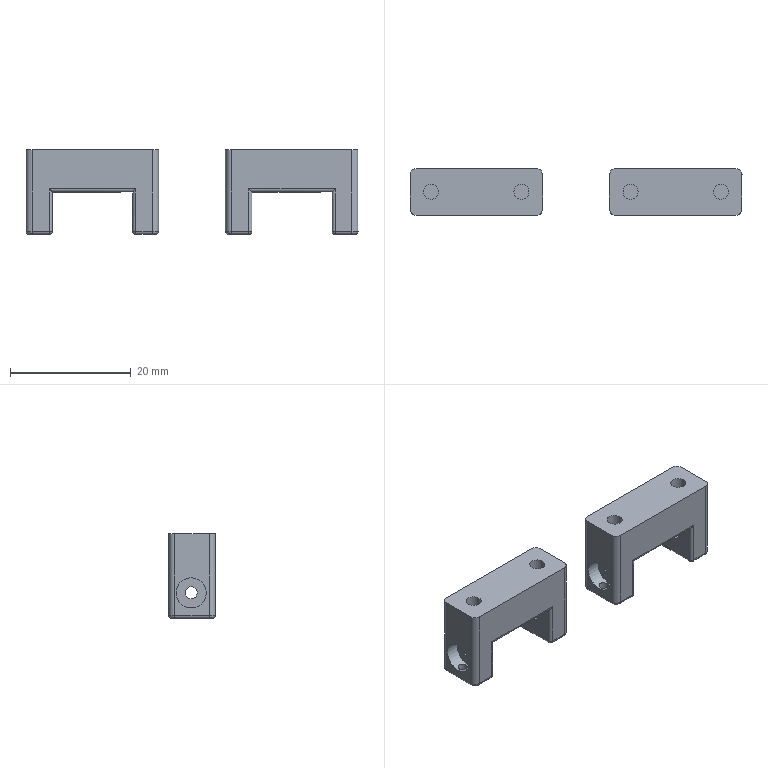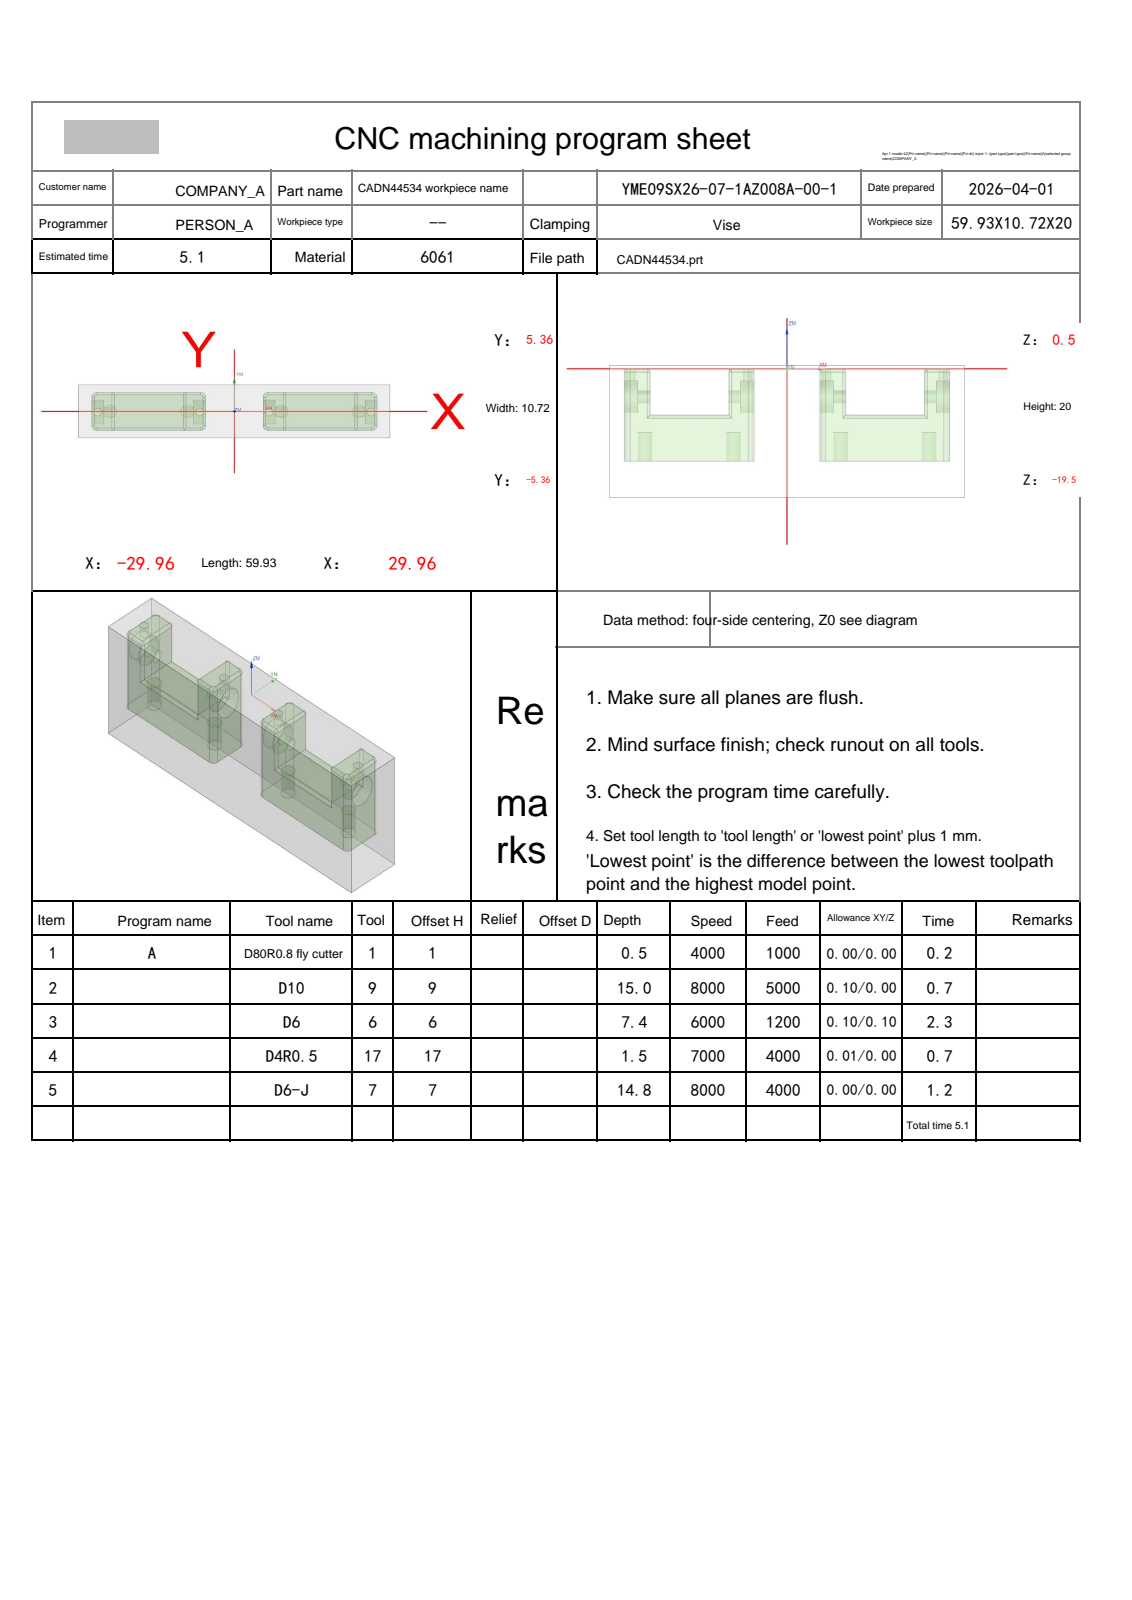NC program | NX | posted by the shop | part box 54.928 x 7.717 x 14 mm
Lines 1616 to 2983 of 13497:
N4 T17 M06
(D4R0.5  D=4. R=0.5 H=17 ce=0.01 di=0.00)
G00 G90 G54 X-28.601 Y-1.585 M03 S7000
G43 H17 Z20.
M08
Z1.5
G01 X-28.598 Y-.024 Z1.418 F4000.
X-28.602 Y2.988 Z1.26
X-28.542 Y3.372 Z1.24
X-28.414 Y3.739 Z1.22
X-28.222 Y4.077 Z1.199
X-27.973 Y4.375 Z1.179
X-27.675 Y4.624 Z1.159
X-27.337 Y4.816 Z1.138
X-26.97 Y4.944 Z1.118
X-26.586 Y5.005 Z1.097
X-23.674 Y5.001 Z.945
X-23.497 Y5.006 Z.936
X-23.368 Y4.999 Z.929
X-23.055 Y4.926 Z.912
X-22.762 Y4.795 Z.895
X-22.499 Y4.608 Z.878
X-22.278 Y4.375 Z.861
X-22.106 Y4.103 Z.845
X-21.99 Y3.804 Z.828
X-21.934 Y3.487 Z.811
Y3.358 Z.804
X-21.944 Y3.286 Z.8
X-21.943 Y-3.286 Z.456
X-21.936 Y-3.436 Z.448
X-21.942 Y-3.565 Z.441
X-22.013 Y-3.88 Z.424
X-22.144 Y-4.175 Z.407
X-22.33 Y-4.439 Z.39
X-22.564 Y-4.662 Z.373
X-22.836 Y-4.835 Z.357
X-23.137 Y-4.952 Z.34
X-23.455 Y-5.008 Z.323
X-23.584 Z.316
X-23.674 Y-5.001 Z.311
X-26.474 Y-5. Z.164
X-26.62 Y-4.999 Z.157
X-26.995 Y-4.938 Z.137
X-27.352 Y-4.812 Z.117
X-27.682 Y-4.625 Z.097
X-27.974 Y-4.383 Z.077
X-28.219 Y-4.093 Z.057
X-28.409 Y-3.765 Z.038
X-28.537 Y-3.408 Z.018
X-28.601 Y-3.034 Z-.002
X-28.603 Y-2.888 Z-.01
G03 X-28.6 Y.376 I-1732.562 J3.264
X-28.602 Y2.841 I-1732.565 J0.0
G01 Y2.844
G02 X-26.441 Y5.004 I2.161 J0.0
G01 X-26.439
X-23.674 Y5.001
X-23.497 Y5.006
G02 X-21.934 Y3.358 I-.087 J-1.648
G01 X-21.944 Y3.286
X-21.943 Y-3.286
X-21.936 Y-3.436
G02 X-23.584 Y-5.008 I-1.648 J.078
G01 X-23.674 Y-5.001
X-26.474 Y-5.
G02 X-28.603 Y-2.888 I.01 J2.14
G01 X-28.613 Y-2.871
Y-2.853
X-28.616 Y-2.146
X-28.618 Y-1.438 Z-.011
Y-1.085
X-28.621 Y-.731
X-28.618 Y-.377
X-28.609 Y-.024
X-28.623 Y.156
X-28.624 Y.336 Z-.012
Y.516
Y.695
X-28.625 Y1.055
X-28.626 Y1.414
X-28.628 Y2.133 Z-.013
X-28.631 Y2.851
Y2.921
X-28.628 Y2.99
X-28.622 Y3.058
X-28.614 Y3.127
X-28.592 Y3.269
X-28.561 Y3.409
X-28.52 Y3.547
X-28.471 Y3.683
X-28.412 Y3.814
X-28.345 Y3.941 Z-.014
X-28.269 Y4.064
X-28.186 Y4.181
X-28.094 Y4.293
X-27.996 Y4.399
X-27.891 Y4.496
X-27.779 Y4.588
X-27.662 Y4.671
X-27.539 Y4.746
X-27.412 Y4.814
X-27.281 Y4.873
X-27.214 Y4.899
X-27.146 Y4.923
X-27.077 Y4.945
X-27.008 Y4.964
X-26.868 Y4.997 Z-.015
X-26.726 Y5.02
X-26.589 Y5.033
X-26.452 Y5.038
X-25.063 Y5.042 Z-.016
X-23.674 Y5.047
X-23.628
X-23.583 Y5.048
X-23.539 Y5.047
X-23.495 Y5.046
X-23.431 Y5.041
X-23.367 Y5.034
X-23.303 Y5.025
X-23.24 Y5.013
X-23.178 Y4.999 Z-.017
X-23.116 Y4.983
X-23.054 Y4.964
X-22.994 Y4.943
X-22.934 Y4.92
X-22.875 Y4.894
X-22.817 Y4.866
X-22.76 Y4.836
X-22.705 Y4.804
X-22.651 Y4.77
X-22.598 Y4.734
X-22.546 Y4.696
X-22.496 Y4.655
X-22.447 Y4.613
X-22.4 Y4.569
X-22.355 Y4.524
X-22.312 Y4.476
X-22.27 Y4.427
X-22.23 Y4.377
X-22.192 Y4.325
X-22.157 Y4.272
X-22.123 Y4.217
X-22.091 Y4.161
X-22.062 Y4.104
X-22.034 Y4.046
X-22.009 Y3.986
X-21.986 Y3.926
X-21.966 Y3.865
X-21.948 Y3.804
X-21.932 Y3.741 Z-.018
X-21.918 Y3.678
X-21.907 Y3.615
X-21.898 Y3.551
X-21.892 Y3.487
X-21.888 Y3.423
X-21.887 Y3.358
Y3.322
X-21.888 Y3.286
X-21.882 Y1.643 Z-.019
X-21.879 Y0.0 Z-.02
X-21.874 Y-1.643
X-21.87 Y-3.286 Z-.021
X-21.869 Y-3.323
Y-3.359
Y-3.399
X-21.871 Y-3.439
X-21.875 Y-3.505
X-21.882 Y-3.569
X-21.89 Y-3.634
X-21.902 Y-3.698
X-21.916 Y-3.762 Z-.022
X-21.933 Y-3.826
X-21.951 Y-3.888
X-21.973 Y-3.95
X-21.996 Y-4.011
X-22.022 Y-4.071
X-22.05 Y-4.13
X-22.081 Y-4.188
X-22.113 Y-4.245
X-22.148 Y-4.3
X-22.184 Y-4.354
X-22.223 Y-4.407
X-22.264 Y-4.458
X-22.307 Y-4.508
X-22.351 Y-4.556
X-22.398 Y-4.602
X-22.446 Y-4.646
X-22.496 Y-4.689
X-22.547 Y-4.729
X-22.6 Y-4.768
X-22.654 Y-4.805
X-22.71 Y-4.839
X-22.767 Y-4.872
X-22.825 Y-4.902
X-22.884 Y-4.93
X-22.944 Y-4.955
X-23.006 Y-4.979
X-23.068 Y-5.
X-23.13 Y-5.018 Z-.023
X-23.194 Y-5.034
X-23.258 Y-5.048
X-23.323 Y-5.06
X-23.388 Y-5.069
X-23.453 Y-5.075
X-23.52 Y-5.079
X-23.587 Y-5.08
X-23.63
X-23.674
X-25.066 Y-5.082 Z-.024
X-26.475 Y-5.084
X-26.547
X-26.619 Y-5.081
X-26.69 Y-5.075
X-26.762 Y-5.065
X-26.833 Y-5.055
X-26.904 Y-5.042 Z-.025
X-26.974 Y-5.027
X-27.044 Y-5.009
X-27.182 Y-4.968
X-27.317 Y-4.917
X-27.448 Y-4.858
X-27.575 Y-4.79
X-27.638 Y-4.754
X-27.698 Y-4.715
X-27.758 Y-4.674
X-27.816 Y-4.631
X-27.928 Y-4.541
X-28.034 Y-4.443
X-28.133 Y-4.338
X-28.225 Y-4.227
X-28.269 Y-4.17
X-28.311 Y-4.111
X-28.35 Y-4.051
X-28.387 Y-3.989 Z-.026
X-28.424 Y-3.927
X-28.457 Y-3.863
X-28.489 Y-3.798
X-28.518 Y-3.732
X-28.57 Y-3.597
X-28.614 Y-3.46
X-28.633 Y-3.39
X-28.649 Y-3.319
X-28.663 Y-3.249
X-28.674 Y-3.177
X-28.684 Y-3.106
X-28.692 Y-3.034
X-28.696 Y-2.962
X-28.693 Y-2.889
X-28.698 Y-2.888
Y-2.87
X-28.699 Y-2.853
X-28.704 Y-1.427 Z-.027
X-28.708 Y-.001 Z-.028
X-28.713 Y1.425 Z-.029
X-28.717 Y2.852 Z-.03
X-28.718 Y2.869
X-28.717 Y2.887
X-28.711 Y3.017 Z-.031
X-28.696 Y3.147
X-28.685 Y3.22
X-28.672 Y3.293
X-28.657 Y3.366
X-28.639 Y3.437
X-28.619 Y3.509
X-28.597 Y3.579
X-28.572 Y3.649
X-28.545 Y3.718
X-28.484 Y3.853
X-28.414 Y3.984
X-28.377 Y4.048
X-28.337 Y4.111
X-28.295 Y4.171
X-28.25 Y4.231
X-28.157 Y4.346 Z-.032
X-28.056 Y4.454
X-28.002 Y4.506
X-27.947 Y4.556
X-27.891 Y4.604
X-27.832 Y4.65
X-27.773 Y4.694
X-27.712 Y4.737
X-27.65 Y4.777
X-27.586 Y4.815
X-27.455 Y4.885
X-27.32 Y4.946
X-27.251 Y4.973
X-27.181 Y4.998
X-27.111 Y5.021 Z-.033
X-27.039 Y5.04
X-26.967 Y5.059
X-26.895 Y5.074
X-26.822 Y5.087
X-26.749 Y5.098
X-26.68 Y5.108
X-26.611 Y5.115
X-26.543 Y5.12
X-26.474 Y5.122
X-26.463
X-26.453
X-25.063 Y5.126 Z-.034
X-23.674 Y5.13 Z-.035
X-23.63 Y5.131
X-23.586
X-23.458 Y5.127
X-23.331 Y5.113
X-23.207 Y5.091
X-23.084 Y5.06
X-22.964 Y5.021 Z-.036
X-22.847 Y4.972
X-22.733 Y4.916
X-22.624 Y4.852
X-22.52 Y4.78
X-22.421 Y4.7
X-22.328 Y4.614
X-22.241 Y4.522
X-22.161 Y4.423
X-22.089 Y4.319
X-22.024 Y4.21 Z-.037
X-21.967 Y4.097
X-21.918 Y3.98
X-21.877 Y3.859
X-21.846 Y3.736
X-21.823 Y3.612
X-21.809 Y3.485
X-21.804 Y3.358
X-21.801 Y1.679 Z-.038
X-21.796 Y0.0 Z-.04
X-21.792 Y-1.679 Z-.041
X-21.787 Y-3.358 Z-.042
X-21.791 Y-3.487
X-21.805 Y-3.614
X-21.827 Y-3.74
X-21.859 Y-3.865 Z-.043
X-21.899 Y-3.987
X-21.948 Y-4.105
X-22.005 Y-4.221
X-22.07 Y-4.331
X-22.143 Y-4.437
X-22.223 Y-4.537
X-22.311 Y-4.631
X-22.405 Y-4.719
X-22.504 Y-4.8
X-22.61 Y-4.874
X-22.72 Y-4.94 Z-.044
X-22.835 Y-4.997
X-22.954 Y-5.047
X-23.076 Y-5.088
X-23.201 Y-5.12
X-23.327 Y-5.143
X-23.457 Y-5.157
X-23.587 Y-5.162
X-23.63 Y-5.16
X-23.673
X-25.065 Y-5.163 Z-.045
X-26.474 Y-5.167 Z-.046
X-26.545 Y-5.165
X-26.616 Y-5.16
X-26.686 Y-5.153 Z-.047
X-26.756 Y-5.144
X-26.83 Y-5.132
X-26.904 Y-5.12
X-26.977 Y-5.104
X-27.05 Y-5.086
X-27.193 Y-5.044
X-27.334 Y-4.993
X-27.471 Y-4.932
X-27.603 Y-4.862
X-27.668 Y-4.824
X-27.731 Y-4.785
X-27.793 Y-4.743
X-27.854 Y-4.698
X-27.971 Y-4.605 Z-.048
X-28.081 Y-4.504
X-28.185 Y-4.395
X-28.281 Y-4.28
X-28.326 Y-4.22
X-28.37 Y-4.16
X-28.412 Y-4.097
X-28.45 Y-4.033
X-28.488 Y-3.968
X-28.523 Y-3.902
X-28.556 Y-3.834
X-28.587 Y-3.766
X-28.641 Y-3.626
X-28.688 Y-3.483 Z-.049
X-28.706 Y-3.411
X-28.724 Y-3.338
X-28.738 Y-3.264
X-28.75 Y-3.19
X-28.762 Y-3.116
X-28.771 Y-3.041
X-28.776 Y-2.966
X-28.779 Y-2.891
X-28.78 Y-2.79
X-28.781 Y-2.689
X-28.785 Y-1.344 Z-.05
X-28.791 Y0.0 Z-.052
X-28.793 Y1.444 Z-.053
X-28.796 Y2.888 Z-.055
X-28.793 Y2.963
X-28.789 Y3.039
X-28.781 Y3.113
X-28.77 Y3.188
X-28.759 Y3.262
X-28.745 Y3.336
X-28.728 Y3.41
X-28.71 Y3.483
X-28.689 Y3.556
X-28.665 Y3.627
X-28.639 Y3.698
X-28.611 Y3.768
X-28.58 Y3.837
X-28.548 Y3.905 Z-.056
X-28.514 Y3.973
X-28.476 Y4.038
X-28.437 Y4.103
X-28.396 Y4.167
X-28.353 Y4.228
X-28.308 Y4.289
X-28.261 Y4.348
X-28.211 Y4.406
X-28.161 Y4.462
X-28.108 Y4.516
X-28.053 Y4.568
X-27.998 Y4.619
X-27.94 Y4.669
X-27.88 Y4.715 Z-.057
X-27.82 Y4.761
X-27.758 Y4.804
X-27.694 Y4.845
X-27.629 Y4.884
X-27.563 Y4.921
X-27.496 Y4.955
X-27.427 Y4.988
X-27.358 Y5.019
X-27.288 Y5.046
X-27.216 Y5.072
X-27.145 Y5.096
X-27.072 Y5.116
X-26.999 Y5.135
X-26.925 Y5.152 Z-.058
X-26.85 Y5.165
X-26.776 Y5.177
X-26.701 Y5.187
X-26.625 Y5.194
X-26.55 Y5.198
X-26.474 Y5.201
X-25.073 Y5.204 Z-.059
X-23.671 Y5.208 Z-.061
X-23.628
X-23.585 Y5.211
X-23.452 Y5.207
X-23.32 Y5.193
X-23.19 Y5.17
X-23.061 Y5.137
X-22.936 Y5.096
X-22.813 Y5.046
X-22.695 Y4.987 Z-.062
X-22.581 Y4.919
X-22.472 Y4.844
X-22.368 Y4.761
X-22.271 Y4.671
X-22.18 Y4.574
X-22.097 Y4.471
X-22.021 Y4.363
X-21.953 Y4.249 Z-.063
X-21.893 Y4.13
X-21.842 Y4.008
X-21.8 Y3.882
X-21.767 Y3.754
X-21.743 Y3.623
X-21.729 Y3.491
X-21.723 Y3.358
X-21.721 Y1.679 Z-.065
X-21.717 Y0.0 Z-.067
X-21.713 Y-1.679 Z-.068
X-21.707 Y-3.358 Z-.07
X-21.711 Y-3.492
X-21.725 Y-3.625
X-21.749 Y-3.757
X-21.782 Y-3.887
X-21.824 Y-4.015
X-21.875 Y-4.139 Z-.071
X-21.934 Y-4.259
X-22.003 Y-4.374
X-22.079 Y-4.485
X-22.163 Y-4.589
X-22.254 Y-4.688
X-22.352 Y-4.78
X-22.457 Y-4.864 Z-.072
X-22.567 Y-4.941
X-22.682 Y-5.01
X-22.802 Y-5.07
X-22.926 Y-5.122
X-23.053 Y-5.165
X-23.184 Y-5.198
X-23.316 Y-5.223
X-23.449 Y-5.237 Z-.073
X-23.584 Y-5.242
X-23.628
X-23.673
X-25.074 Y-5.245 Z-.074
X-26.474 Y-5.249 Z-.075
X-26.629 Y-5.243 Z-.076
X-26.782 Y-5.228
X-26.859 Y-5.216
X-26.935 Y-5.203
X-27.01 Y-5.186
X-27.085 Y-5.168
X-27.233 Y-5.123
X-27.378 Y-5.069
X-27.519 Y-5.005
X-27.656 Y-4.933 Z-.077
X-27.723 Y-4.894
X-27.788 Y-4.852
X-27.852 Y-4.808
X-27.914 Y-4.762
X-27.976 Y-4.715
X-28.035 Y-4.665
X-28.093 Y-4.613
X-28.149 Y-4.56
X-28.203 Y-4.504
X-28.255 Y-4.447
X-28.306 Y-4.389
X-28.355 Y-4.328
X-28.401 Y-4.266 Z-.078
X-28.446 Y-4.203
X-28.489 Y-4.138
X-28.529 Y-4.072
X-28.568 Y-4.005
X-28.604 Y-3.936
X-28.637 Y-3.866
X-28.669 Y-3.796
X-28.725 Y-3.651
X-28.772 Y-3.504
X-28.792 Y-3.429
X-28.81 Y-3.353
X-28.825 Y-3.277 Z-.079
X-28.836 Y-3.201
X-28.847 Y-3.124
X-28.855 Y-3.047
X-28.859 Y-2.97
X-28.86 Y-2.892
X-28.863 Y-2.791
Y-2.689
X-28.861 Y-1.295 Z-.081
X-28.864 Y.1 Z-.082
X-28.869 Y1.494 Z-.084
X-28.877 Y2.888 Z-.086
X-28.871 Y3.032
X-28.857 Y3.176
X-28.846 Y3.247
X-28.834 Y3.318
X-28.819 Y3.389
X-28.802 Y3.459
X-28.763 Y3.598
X-28.715 Y3.734 Z-.087
X-28.659 Y3.867
X-28.595 Y3.996
X-28.523 Y4.122
X-28.445 Y4.243
X-28.359 Y4.359
X-28.266 Y4.469 Z-.088
X-28.217 Y4.523
X-28.167 Y4.575
X-28.115 Y4.625
X-28.061 Y4.673
X-27.95 Y4.766
X-27.834 Y4.852
X-27.712 Y4.93
X-27.587 Y5.002 Z-.089
X-27.457 Y5.065
X-27.323 Y5.121
X-27.255 Y5.146
X-27.187 Y5.169
X-27.117 Y5.189
X-27.047 Y5.207
X-26.977 Y5.225
X-26.906 Y5.239
X-26.835 Y5.251
X-26.763 Y5.261 Z-.09
X-26.619 Y5.275
X-26.474 Y5.281
X-25.073 Y5.285 Z-.091
X-23.672 Y5.288 Z-.093
X-23.628
X-23.585 Y5.29
X-23.516 Y5.289
X-23.446 Y5.285
X-23.377 Y5.279
X-23.309 Y5.271 Z-.094
X-23.241 Y5.26
X-23.173 Y5.247
X-23.106 Y5.231
X-23.039 Y5.213
X-22.973 Y5.192
X-22.908 Y5.169
X-22.844 Y5.144
X-22.781 Y5.117
X-22.718 Y5.087
X-22.657 Y5.056
X-22.597 Y5.022
X-22.538 Y4.985
X-22.481 Y4.947 Z-.095
X-22.425 Y4.907
X-22.37 Y4.865
X-22.317 Y4.821
X-22.265 Y4.775
X-22.216 Y4.727
X-22.167 Y4.677
X-22.121 Y4.626
X-22.077 Y4.573
X-22.034 Y4.518
X-21.994 Y4.462
X-21.955 Y4.405
X-21.919 Y4.346
X-21.884 Y4.286 Z-.096
X-21.852 Y4.225
X-21.822 Y4.163
X-21.794 Y4.1
X-21.769 Y4.035
X-21.746 Y3.97
X-21.725 Y3.904
X-21.706 Y3.838
X-21.69 Y3.77
X-21.677 Y3.702
X-21.665 Y3.634
X-21.657 Y3.566
X-21.65 Y3.497 Z-.097
X-21.646 Y3.428
X-21.645 Y3.358
X-21.643 Y1.679 Z-.099
X-21.639 Y0.0 Z-.101
X-21.635 Y-1.679 Z-.102
X-21.629 Y-3.358 Z-.104
X-21.63 Y-3.428
X-21.634 Y-3.498 Z-.105
X-21.64 Y-3.567
X-21.649 Y-3.637
X-21.659 Y-3.705
X-21.673 Y-3.774
X-21.689 Y-3.842
X-21.707 Y-3.909
X-21.728 Y-3.976
X-21.751 Y-4.042
X-21.776 Y-4.107
X-21.804 Y-4.171
X-21.834 Y-4.234
X-21.866 Y-4.296 Z-.106
X-21.901 Y-4.357
X-21.937 Y-4.416
X-21.976 Y-4.475
X-22.017 Y-4.531
X-22.059 Y-4.587
X-22.104 Y-4.64
X-22.151 Y-4.693
X-22.199 Y-4.743
X-22.249 Y-4.792
X-22.301 Y-4.838
X-22.355 Y-4.883
X-22.41 Y-4.926
X-22.467 Y-4.968 Z-.107
X-22.525 Y-5.006
X-22.584 Y-5.043
X-22.645 Y-5.078
X-22.707 Y-5.111
X-22.77 Y-5.141
X-22.834 Y-5.169
X-22.899 Y-5.195
X-22.965 Y-5.218
X-23.032 Y-5.239
X-23.099 Y-5.258
X-23.167 Y-5.274
X-23.236 Y-5.288 Z-.108
X-23.305 Y-5.299
X-23.374 Y-5.308
X-23.444 Y-5.315
X-23.514 Y-5.319
X-23.584 Y-5.32
X-23.628 Y-5.318
X-23.673
X-25.074 Y-5.321 Z-.11
X-26.475 Y-5.325 Z-.111
X-26.554 Y-5.322
X-26.634 Y-5.318
X-26.713 Y-5.31 Z-.112
X-26.792 Y-5.3
X-26.871 Y-5.288
X-26.95 Y-5.275
X-27.027 Y-5.257
X-27.105 Y-5.238
X-27.181 Y-5.217
X-27.257 Y-5.192
X-27.332 Y-5.165
X-27.407 Y-5.136
X-27.48 Y-5.104
X-27.552 Y-5.071 Z-.113
X-27.623 Y-5.035
X-27.693 Y-4.996
X-27.761 Y-4.955
X-27.829 Y-4.913
X-27.894 Y-4.867
X-27.959 Y-4.82
X-28.022 Y-4.771
X-28.083 Y-4.72
X-28.142 Y-4.666
X-28.2 Y-4.612
X-28.256 Y-4.554 Z-.114
X-28.31 Y-4.495
X-28.362 Y-4.435
X-28.412 Y-4.373
X-28.46 Y-4.309
X-28.507 Y-4.244
X-28.55 Y-4.178
X-28.591 Y-4.109
X-28.632 Y-4.04
X-28.669 Y-3.97
X-28.703 Y-3.898
X-28.736 Y-3.825 Z-.115
X-28.766 Y-3.751
X-28.794 Y-3.676
X-28.82 Y-3.601
X-28.843 Y-3.524
X-28.862 Y-3.447
X-28.881 Y-3.369
X-28.896 Y-3.291
X-28.909 Y-3.212
X-28.92 Y-3.133
X-28.928 Y-3.053
X-28.935 Y-2.974 Z-.116
X-28.937 Y-2.894
X-28.939 Y-2.852
Y-2.81
Y-2.75
Y-2.689
X-28.943 Y-1.344 Z-.118
X-28.946 Y0.0 Z-.119
X-28.95 Y1.344 Z-.121
X-28.953 Y2.689 Z-.123
X-28.954 Y2.75
X-28.953 Y2.811
X-28.954 Y2.849
X-28.953 Y2.888
X-28.945 Y3.036
X-28.928 Y3.184 Z-.124
X-28.918 Y3.258
X-28.905 Y3.331
X-28.89 Y3.404
X-28.872 Y3.476
X-28.832 Y3.619
X-28.783 Y3.759
X-28.725 Y3.896
X-28.659 Y4.03 Z-.125
X-28.585 Y4.159
X-28.504 Y4.284
X-28.416 Y4.404
X-28.32 Y4.517
X-28.27 Y4.573 Z-.126
X-28.218 Y4.626
X-28.164 Y4.678
X-28.109 Y4.728
X-27.995 Y4.823
X-27.875 Y4.912
X-27.749 Y4.992
X-27.62 Y5.066 Z-.127
X-27.486 Y5.131
X-27.348 Y5.189
X-27.278 Y5.214
X-27.208 Y5.238
X-27.136 Y5.259
X-27.064 Y5.278
X-26.919 Y5.31 Z-.128
X-26.771 Y5.333
X-26.623 Y5.35
X-26.459 Y5.358
X-25.065 Y5.361 Z-.13
X-23.672 Y5.364 Z-.132
X-23.628 Y5.365
X-23.584 Y5.364
X-23.453 Y5.361
X-23.322 Y5.348
X-23.192 Y5.327
X-23.064 Y5.297 Z-.133
X-22.938 Y5.26
X-22.815 Y5.214
X-22.696 Y5.16
X-22.58 Y5.098
X-22.468 Y5.029
X-22.361 Y4.952 Z-.134
X-22.259 Y4.869
X-22.163 Y4.78
X-22.073 Y4.684
X-21.989 Y4.582
X-21.912 Y4.475
X-21.842 Y4.364 Z-.135
X-21.78 Y4.248
X-21.725 Y4.128
X-21.679 Y4.005
X-21.64 Y3.879
X-21.61 Y3.751 Z-.136
X-21.588 Y3.621
X-21.575 Y3.49
X-21.57 Y3.358
X-21.567 Y1.679 Z-.138
X-21.563 Y0.0 Z-.14
X-21.56 Y-1.679 Z-.143
X-21.556 Y-3.358 Z-.145
X-21.56 Y-3.491
X-21.573 Y-3.623
X-21.594 Y-3.754
X-21.624 Y-3.883
X-21.662 Y-4.011 Z-.146
X-21.709 Y-4.135
X-21.763 Y-4.256
X-21.826 Y-4.373
X-21.895 Y-4.486
X-21.973 Y-4.595
X-22.057 Y-4.698 Z-.147
X-22.147 Y-4.795
X-22.244 Y-4.886
X-22.347 Y-4.97
X-22.455 Y-5.048
X-22.568 Y-5.119 Z-.148
X-22.685 Y-5.182
X-22.806 Y-5.237
X-22.93 Y-5.284
X-23.057 Y-5.323
X-23.187 Y-5.353
X-23.318 Y-5.375 Z-.149
X-23.452 Y-5.389
X-23.586 Y-5.393
X-23.63
X-23.673
X-25.066 Y-5.396 Z-.151
X-26.474 Y-5.399 Z-.153
X-26.626 Y-5.393
X-26.777 Y-5.379
X-26.927 Y-5.356
X-27.075 Y-5.324
X-27.221 Y-5.284 Z-.154
X-27.364 Y-5.235
X-27.505 Y-5.177
X-27.642 Y-5.111
X-27.774 Y-5.037
X-27.902 Y-4.956 Z-.155
X-28.025 Y-4.866
X-28.142 Y-4.769
X-28.198 Y-4.718
X-28.254 Y-4.666
X-28.307 Y-4.612
X-28.358 Y-4.556
X-28.457 Y-4.44 Z-.156
X-28.548 Y-4.319
X-28.631 Y-4.192
X-28.708 Y-4.061
X-28.775 Y-3.924
X-28.835 Y-3.785 Z-.157
X-28.887 Y-3.642
X-28.929 Y-3.496
X-28.947 Y-3.422
X-28.964 Y-3.348
X-28.977 Y-3.273
X-28.988 Y-3.198
X-28.998 Y-3.123
X-29.004 Y-3.047 Z-.158
X-29.009 Y-2.971
X-29.011 Y-2.895
X-29.013 Y-2.853
Y-2.81
Y-2.75
Y-2.689
X-29.016 Y-1.344 Z-.16
X-29.019 Y0.0 Z-.162
X-29.023 Y1.344 Z-.164
X-29.025 Y2.689 Z-.166
X-29.026 Y2.75
Y2.811
Y2.849
X-29.025 Y2.887
X-29.021 Y3.005 Z-.167
X-29.012 Y3.123
X-28.991 Y3.279
X-28.961 Y3.432
X-28.943 Y3.509
X-28.922 Y3.584
X-28.899 Y3.659 Z-.168
X-28.873 Y3.733
X-28.846 Y3.807
X-28.816 Y3.879
X-28.783 Y3.951
X-28.749 Y4.021
X-28.674 Y4.159
X-28.591 Y4.292 Z-.169
X-28.499 Y4.42
X-28.4 Y4.541
X-28.348 Y4.6
X-28.294 Y4.657
X-28.238 Y4.712
X-28.18 Y4.765 Z-.17
X-28.122 Y4.818
X-28.061 Y4.868
X-27.998 Y4.915
X-27.935 Y4.962
X-27.804 Y5.048
X-27.668 Y5.127 Z-.171
X-27.526 Y5.196
X-27.382 Y5.257
X-27.308 Y5.284
X-27.233 Y5.309
X-27.158 Y5.332
X-27.082 Y5.351
X-27.005 Y5.37 Z-.172
X-26.928 Y5.386
X-26.851 Y5.398
X-26.773 Y5.41
X-26.624 Y5.423
X-26.474 Y5.429
X-25.073 Y5.432 Z-.175
X-23.672 Y5.435 Z-.177
X-23.628 Y5.436
X-23.585
X-23.448 Y5.432
X-23.313 Y5.419
X-23.178 Y5.397
X-23.046 Y5.366 Z-.178
X-22.916 Y5.327
X-22.788 Y5.279
X-22.664 Y5.223
X-22.544 Y5.16
X-22.428 Y5.088 Z-.179
X-22.317 Y5.009
X-22.212 Y4.923
X-22.112 Y4.83
X-22.019 Y4.731
X-21.932 Y4.626 Z-.18
X-21.853 Y4.515
X-21.781 Y4.399
X-21.716 Y4.279
X-21.66 Y4.155
X-21.611 Y4.028 Z-.181
X-21.571 Y3.898
X-21.54 Y3.765
X-21.518 Y3.63
X-21.504 Y3.495
X-21.499 Y3.358 Z-.182
X-21.496 Y1.679 Z-.184
X-21.493 Y0.0 Z-.187
X-21.49 Y-1.679 Z-.189
X-21.485 Y-3.358 Z-.192
X-21.489 Y-3.496
X-21.503 Y-3.632
X-21.525 Y-3.768
X-21.556 Y-3.902 Z-.193
X-21.595 Y-4.033
X-21.643 Y-4.162
X-21.7 Y-4.287
X-21.765 Y-4.409
X-21.837 Y-4.526 Z-.194
X-21.917 Y-4.638
X-22.004 Y-4.744
X-22.098 Y-4.845
X-22.198 Y-4.939
X-22.304 Y-5.026 Z-.195
X-22.416 Y-5.107
X-22.532 Y-5.18
X-22.654 Y-5.245
X-22.779 Y-5.302
X-22.908 Y-5.351 Z-.196
X-23.039 Y-5.391
X-23.173 Y-5.422
X-23.309 Y-5.445
X-23.447 Y-5.459
X-23.586 Y-5.463 Z-.197
X-23.629 Y-5.462
X-23.673
X-25.066 Y-5.464 Z-.199
X-26.474 Y-5.467 Z-.201
X-26.623 Y-5.462
X-26.771 Y-5.449
X-26.848 Y-5.438 Z-.202
X-26.926 Y-5.427
X-27.002 Y-5.412
X-27.078 Y-5.394
X-27.154 Y-5.375
X-27.23 Y-5.354
X-27.304 Y-5.329
X-27.378 Y-5.303
X-27.523 Y-5.244 Z-.203
X-27.664 Y-5.177
X-27.801 Y-5.101
X-27.933 Y-5.018
X-28.06 Y-4.925 Z-.204
X-28.181 Y-4.826
X-28.239 Y-4.774
X-28.296 Y-4.72
X-28.351 Y-4.665
X-28.404 Y-4.607
X-28.456 Y-4.549
X-28.506 Y-4.488
X-28.554 Y-4.426 Z-.205
X-28.6 Y-4.363
X-28.686 Y-4.232
X-28.766 Y-4.097
X-28.835 Y-3.957
X-28.898 Y-3.813 Z-.206
X-28.925 Y-3.74
X-28.951 Y-3.666
X-28.974 Y-3.591
X-28.994 Y-3.515
X-29.013 Y-3.439
X-29.03 Y-3.363
X-29.044 Y-3.286
X-29.055 Y-3.208 Z-.207
X-29.072 Y-3.053
X-29.08 Y-2.896
X-29.083 Y-1.448 Z-.21
X-29.089 Y1.444 Z-.214
X-29.092 Y2.888 Z-.217
X-29.085 Y3.045
X-29.07 Y3.201
X-29.058 Y3.279 Z-.218
X-29.045 Y3.357
X-29.029 Y3.434
X-29.01 Y3.51
X-28.991 Y3.586
X-28.968 Y3.662
X-28.942 Y3.736
X-28.916 Y3.81
X-28.854 Y3.955 Z-.219
X-28.785 Y4.096
X-28.707 Y4.233
X-28.621 Y4.365 Z-.22
X-28.575 Y4.428
X-28.528 Y4.491
X-28.478 Y4.552
X-28.426 Y4.612
X-28.373 Y4.67
X-28.318 Y4.727
X-28.261 Y4.781
X-28.203 Y4.834 Z-.221
X-28.082 Y4.935
X-27.955 Y5.029
X-27.823 Y5.113
X-27.686 Y5.192 Z-.222
X-27.544 Y5.261
X-27.399 Y5.321
X-27.325 Y5.348
X-27.25 Y5.373
X-27.175 Y5.396 Z-.223
X-27.098 Y5.415
X-27.022 Y5.434
X-26.944 Y5.45
X-26.867 Y5.462
X-26.789 Y5.474
X-26.632 Y5.489 Z-.224
X-26.474 Y5.495
X-26.374
X-26.274 Y5.496
X-24.973 Y5.499 Z-.226
X-23.672 Y5.501 Z-.229
X-23.628
X-23.584 Y5.505
X-23.443 Y5.5
X-23.304 Y5.487
X-23.165 Y5.464
X-23.028 Y5.433 Z-.23
X-22.893 Y5.392
X-22.762 Y5.343
X-22.634 Y5.285
X-22.509 Y5.219 Z-.231
X-22.39 Y5.145
X-22.275 Y5.063
X-22.167 Y4.974
X-22.064 Y4.879 Z-.232
X-21.967 Y4.776
X-21.878 Y4.667
X-21.796 Y4.553
X-21.721 Y4.434 Z-.233
X-21.654 Y4.31
X-21.596 Y4.182
X-21.546 Y4.05
X-21.505 Y3.915 Z-.234
X-21.473 Y3.778
X-21.449 Y3.639
X-21.436 Y3.499
X-21.43 Y3.358
X-21.431 Y1.679 Z-.237
X-21.427 Y0.0 Z-.24
X-21.424 Y-1.679 Z-.243
X-21.417 Y-3.358 Z-.246
X-21.422 Y-3.5
X-21.435 Y-3.641
X-21.458 Y-3.781 Z-.247
X-21.49 Y-3.919
X-21.531 Y-4.055
X-21.581 Y-4.188
X-21.639 Y-4.317 Z-.248
X-21.706 Y-4.443
X-21.78 Y-4.563
X-21.863 Y-4.679
X-21.953 Y-4.789 Z-.249
X-22.05 Y-4.893
X-22.153 Y-4.99
X-22.263 Y-5.08
X-22.378 Y-5.163 Z-.25
X-22.498 Y-5.238
X-22.624 Y-5.306
X-22.753 Y-5.364
X-22.886 Y-5.415
X-23.022 Y-5.456 Z-.251
X-23.16 Y-5.489
X-23.3 Y-5.512
X-23.442 Y-5.527
X-23.584 Y-5.531 Z-.252
X-23.628 Y-5.529
X-23.673
X-25.074 Y-5.532 Z-.254
X-26.474 Y-5.535 Z-.257
X-26.634 Y-5.529
X-26.793 Y-5.515
X-26.951 Y-5.491
X-27.107 Y-5.457 Z-.258
X-27.185 Y-5.437
X-27.261 Y-5.415
X-27.337 Y-5.389
X-27.412 Y-5.363
X-27.56 Y-5.302
X-27.705 Y-5.233 Z-.259
X-27.844 Y-5.154
X-27.979 Y-5.069
X-28.108 Y-4.974 Z-.26
X-28.232 Y-4.872
X-28.291 Y-4.819
X-28.349 Y-4.764
X-28.405 Y-4.707
X-28.459 Y-4.648
X-28.512 Y-4.588 Z-.261
X-28.563 Y-4.526
X-28.612 Y-4.462
X-28.659 Y-4.398
X-28.747 Y-4.264
X-28.828 Y-4.126
X-28.899 Y-3.982 Z-.262
X-28.962 Y-3.835
X-29.016 Y-3.684
X-29.061 Y-3.53 Z-.263
X-29.08 Y-3.453
X-29.097 Y-3.375
X-29.111 Y-3.296
X-29.123 Y-3.216
X-29.134 Y-3.137
X-29.14 Y-3.057
X-29.145 Y-2.977 Z-.264
X-29.147 Y-2.897
X-29.152 Y-1.449 Z-.266
X-29.155 Y0.0 Z-.269
X-29.157 Y1.444 Z-.271
X-29.16 Y2.888 Z-.274
X-29.153 Y3.049
X-29.137 Y3.21
X-29.126 Y3.29 Z-.275
X-29.112 Y3.369
X-29.096 Y3.448
X-29.076 Y3.526
X-29.056 Y3.605
X-29.033 Y3.682
X-29.007 Y3.758
X-28.979 Y3.834 Z-.276
X-28.916 Y3.983
X-28.845 Y4.128
X-28.765 Y4.268
X-28.677 Y4.404 Z-.277
X-28.629 Y4.469
X-28.581 Y4.534
X-28.53 Y4.596
X-28.477 Y4.657
X-28.422 Y4.717
X-28.366 Y4.775 Z-.278
X-28.308 Y4.831
X-28.248 Y4.885
X-28.124 Y4.989
X-27.994 Y5.085
X-27.858 Y5.172 Z-.279
X-27.717 Y5.252
X-27.572 Y5.323
X-27.423 Y5.385 Z-.28
X-27.346 Y5.412
X-27.27 Y5.438
X-27.193 Y5.461
X-27.114 Y5.481
X-27.036 Y5.501
X-26.956 Y5.517
X-26.877 Y5.53 Z-.281
X-26.797 Y5.541
X-26.636 Y5.557
X-26.474 Y5.563
X-26.374 Y5.564 Z-.282
X-26.274
X-24.974 Y5.566 Z-.284
X-23.674 Y5.569 Z-.286
X-23.629
X-23.584
X-23.439 Y5.564 Z-.287
X-23.295 Y5.55
X-23.152 Y5.527
X-23.011 Y5.494
X-22.873 Y5.453 Z-.288
X-22.737 Y5.402
X-22.605 Y5.342
X-22.478 Y5.274 Z-.289
X-22.355 Y5.198
X-22.237 Y5.114
X-22.125 Y5.022
X-22.019 Y4.924 Z-.29
X-21.919 Y4.818
X-21.827 Y4.706
X-21.743 Y4.589
X-21.666 Y4.466 Z-.291
X-21.597 Y4.338
X-21.537 Y4.206
X-21.486 Y4.07
X-21.444 Y3.932 Z-.292
X-21.411 Y3.791
X-21.387 Y3.648
X-21.372 Y3.503
X-21.367 Y3.358 Z-.293
X-21.365 Y1.679 Z-.296
X-21.362 Y0.0 Z-.299
X-21.359 Y-1.679 Z-.302
X-21.356 Y-3.358 Z-.305
X-21.36 Y-3.504
X-21.374 Y-3.649
X-21.398 Y-3.793
X-21.431 Y-3.935 Z-.306
X-21.473 Y-4.075
X-21.524 Y-4.212
X-21.584 Y-4.345
X-21.652 Y-4.473 Z-.307
X-21.729 Y-4.598
X-21.814 Y-4.716
X-21.906 Y-4.829
X-22.006 Y-4.936 Z-.308
X-22.112 Y-5.036
X-22.225 Y-5.129
X-22.344 Y-5.214
X-22.468 Y-5.291 Z-.309
X-22.596 Y-5.361
X-22.729 Y-5.421
X-22.866 Y-5.473
X-23.006 Y-5.515 Z-.31
X-23.148 Y-5.549
X-23.292 Y-5.573
X-23.438 Y-5.588
X-23.584 Y-5.593 Z-.311
X-23.629
X-23.674 Y-5.592
X-25.074 Y-5.594 Z-.313
X-26.474 Y-5.597 Z-.316
X-26.638 Y-5.591
X-26.8 Y-5.576
X-26.881 Y-5.564 Z-.317
X-26.962 Y-5.552
X-27.042 Y-5.536
X-27.122 Y-5.517
X-27.201 Y-5.496
X-27.28 Y-5.474
X-27.357 Y-5.448
X-27.434 Y-5.42 Z-.318
X-27.585 Y-5.358
X-27.733 Y-5.287
X-27.875 Y-5.206
X-28.014 Y-5.119 Z-.319
X-28.146 Y-5.022
X-28.272 Y-4.918
X-28.333 Y-4.863
X-28.392 Y-4.807 Z-.32
X-28.449 Y-4.749
X-28.505 Y-4.688
X-28.559 Y-4.627
X-28.611 Y-4.564
X-28.66 Y-4.499
X-28.709 Y-4.433
X-28.799 Y-4.296 Z-.321
X-28.881 Y-4.154
X-28.954 Y-4.008
X-29.019 Y-3.857 Z-.322
X-29.047 Y-3.78
X-29.074 Y-3.703
X-29.098 Y-3.625
X-29.119 Y-3.546
X-29.139 Y-3.466
X-29.157 Y-3.386
X-29.171 Y-3.306 Z-.323
X-29.183 Y-3.225
X-29.194 Y-3.143
X-29.201 Y-3.062
X-29.205 Y-2.98
X-29.206 Y-2.898
X-29.211 Y-1.449 Z-.326
X-29.213 Y0.0 Z-.329
X-29.216 Y1.444 Z-.332
X-29.218 Y2.888 Z-.335
X-29.215 Y2.97
X-29.211 Y3.053
X-29.205 Y3.135
X-29.195 Y3.217
X-29.183 Y3.298
X-29.169 Y3.38 Z-.336
X-29.152 Y3.46
X-29.132 Y3.54
X-29.112 Y3.62
X-29.088 Y3.699
X-29.061 Y3.777
X-29.033 Y3.855
X-29.002 Y3.931 Z-.337
X-28.968 Y4.007
X-28.933 Y4.081
X-28.896 Y4.155
X-28.856 Y4.227
X-28.814 Y4.298
X-28.771 Y4.368 Z-.338
X-28.724 Y4.436
X-28.676 Y4.503
X-28.626 Y4.569
X-28.574 Y4.633
X-28.52 Y4.695
X-28.464 Y4.756 Z-.339
X-28.407 Y4.815
X-28.347 Y4.872
X-28.286 Y4.928
X-28.224 Y4.982
X-28.159 Y5.033
X-28.093 Y5.083 Z-.34
X-28.026 Y5.131
X-27.958 Y5.177
X-27.887 Y5.22
X-27.817 Y5.263
X-27.744 Y5.302
X-27.67 Y5.339
X-27.596 Y5.374 Z-.341
X-27.52 Y5.408
X-27.443 Y5.438
X-27.365 Y5.466
X-27.287 Y5.492
X-27.208 Y5.516
X-27.128 Y5.536 Z-.342
X-27.048 Y5.556
X-26.967 Y5.572
X-26.885 Y5.586
X-26.804 Y5.598
X-26.722 Y5.607
X-26.639 Y5.613 Z-.343
X-26.557 Y5.617
X-26.474 Y5.62
X-25.074 Y5.622 Z-.346
X-23.674 Y5.624 Z-.348
X-23.629
X-23.584 Y5.627
X-23.435 Y5.622 Z-.349
X-23.288 Y5.608
X-23.141 Y5.584
X-22.996 Y5.55 Z-.35
X-22.854 Y5.507
X-22.715 Y5.456
X-22.58 Y5.394
X-22.449 Y5.325 Z-.351
X-22.322 Y5.246
X-22.201 Y5.16